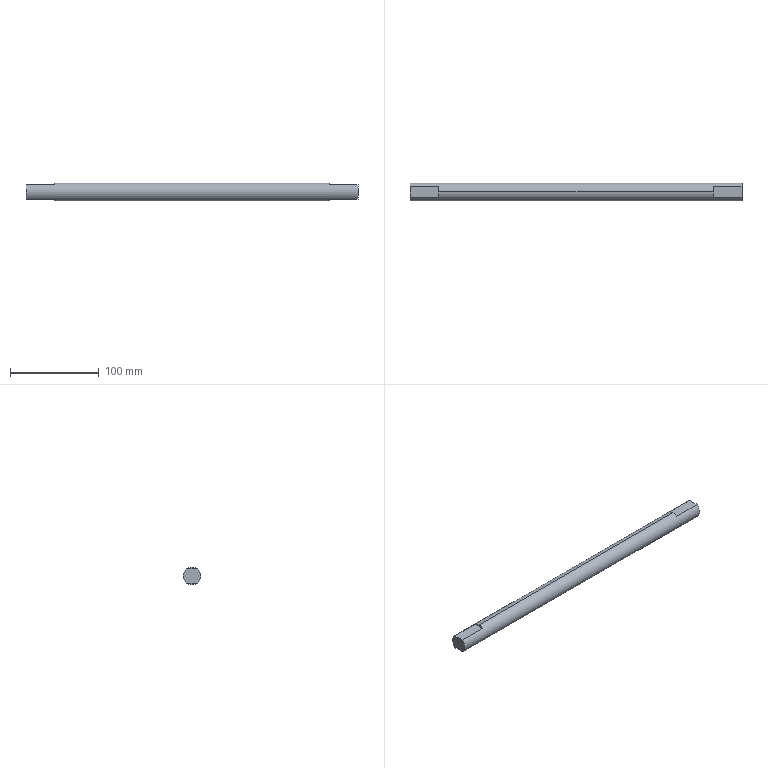Part | SolidWorks | features ICE 3, Extrusion 1, HoleWzd 1 | 1 solid | 12 faces | box 374 x 20 x 20 mm | volume 115370 mm3 | plane 10 | cylinder 2 | commonest cylinder face diameters 20 x2
STEP:
#1=CARTESIAN_POINT('',(341.5,6.,-8.));
#2=VERTEX_POINT('',#1);
#3=CARTESIAN_POINT('',(341.5,0.,-10.));
#4=VERTEX_POINT('',#3);
#5=CARTESIAN_POINT('',(341.5,0.,0.));
#6=DIRECTION('',(-1.,0.,0.));
#7=DIRECTION('',(0.,0.,1.));
#8=AXIS2_PLACEMENT_3D('',#5,#6,#7);
#9=CIRCLE('',#8,10.);
#10=EDGE_CURVE('',#2,#4,#9,.T.);
#11=ORIENTED_EDGE('',*,*,#10,.T.);
#12=CARTESIAN_POINT('',(32.5,0.,-10.));
#13=VERTEX_POINT('',#12);
#14=CARTESIAN_POINT('',(374.,0.,-10.));
#15=DIRECTION('',(-1.,0.,0.));
#16=VECTOR('',#15,1000.);
#17=LINE('',#14,#16);
#18=EDGE_CURVE('',#4,#13,#17,.T.);
#19=ORIENTED_EDGE('',*,*,#18,.T.);
#20=CARTESIAN_POINT('',(32.5,6.,-8.));
#21=VERTEX_POINT('',#20);
#22=CARTESIAN_POINT('',(32.5,0.,0.));
#23=DIRECTION('',(1.,0.,0.));
#24=DIRECTION('',(0.,1.,0.));
#25=AXIS2_PLACEMENT_3D('',#22,#23,#24);
#26=CIRCLE('',#25,10.);
#27=EDGE_CURVE('',#13,#21,#26,.T.);
#28=ORIENTED_EDGE('',*,*,#27,.T.);
#29=CARTESIAN_POINT('',(0.,6.,-8.));
#30=VERTEX_POINT('',#29);
#31=CARTESIAN_POINT('',(374.,6.,-8.));
#32=DIRECTION('',(-1.,0.,0.));
#33=VECTOR('',#32,1000.);
#34=LINE('',#31,#33);
#35=EDGE_CURVE('',#21,#30,#34,.T.);
#36=ORIENTED_EDGE('',*,*,#35,.T.);
#37=CARTESIAN_POINT('',(0.,6.,8.));
#38=VERTEX_POINT('',#37);
#39=CARTESIAN_POINT('',(0.,0.,0.));
#40=DIRECTION('',(1.,0.,0.));
#41=DIRECTION('',(0.,0.,-1.));
#42=AXIS2_PLACEMENT_3D('',#39,#40,#41);
#43=CIRCLE('',#42,10.);
#44=EDGE_CURVE('',#30,#38,#43,.T.);
#45=ORIENTED_EDGE('',*,*,#44,.T.);
#46=CARTESIAN_POINT('',(32.5,6.,8.));
#47=VERTEX_POINT('',#46);
#48=CARTESIAN_POINT('',(374.,6.,8.));
#49=DIRECTION('',(-1.,0.,0.));
#50=VECTOR('',#49,1000.);
#51=LINE('',#48,#50);
#52=EDGE_CURVE('',#47,#38,#51,.T.);
#53=ORIENTED_EDGE('',*,*,#52,.F.);
#54=CARTESIAN_POINT('',(32.5,0.,10.));
#55=VERTEX_POINT('',#54);
#56=CARTESIAN_POINT('',(32.5,0.,0.));
#57=DIRECTION('',(-1.,0.,0.));
#58=DIRECTION('',(0.,-1.,0.));
#59=AXIS2_PLACEMENT_3D('',#56,#57,#58);
#60=CIRCLE('',#59,10.);
#61=EDGE_CURVE('',#55,#47,#60,.T.);
#62=ORIENTED_EDGE('',*,*,#61,.F.);
#63=CARTESIAN_POINT('',(341.5,0.,10.));
#64=VERTEX_POINT('',#63);
#65=CARTESIAN_POINT('',(374.,0.,10.));
#66=DIRECTION('',(-1.,0.,0.));
#67=VECTOR('',#66,1000.);
#68=LINE('',#65,#67);
#69=EDGE_CURVE('',#64,#55,#68,.T.);
#70=ORIENTED_EDGE('',*,*,#69,.F.);
#71=CARTESIAN_POINT('',(341.5,6.,8.));
#72=VERTEX_POINT('',#71);
#73=CARTESIAN_POINT('',(341.5,0.,0.));
#74=DIRECTION('',(1.,0.,0.));
#75=DIRECTION('',(0.,0.,-1.));
#76=AXIS2_PLACEMENT_3D('',#73,#74,#75);
#77=CIRCLE('',#76,10.);
#78=EDGE_CURVE('',#72,#64,#77,.T.);
#79=ORIENTED_EDGE('',*,*,#78,.F.);
#80=CARTESIAN_POINT('',(374.,6.,8.));
#81=VERTEX_POINT('',#80);
#82=CARTESIAN_POINT('',(374.,6.,8.));
#83=DIRECTION('',(-1.,0.,0.));
#84=VECTOR('',#83,1000.);
#85=LINE('',#82,#84);
#86=EDGE_CURVE('',#81,#72,#85,.T.);
#87=ORIENTED_EDGE('',*,*,#86,.F.);
#88=CARTESIAN_POINT('',(374.,6.,-8.));
#89=VERTEX_POINT('',#88);
#90=CARTESIAN_POINT('',(374.,0.,0.));
#91=DIRECTION('',(1.,0.,0.));
#92=DIRECTION('',(0.,0.,-1.));
#93=AXIS2_PLACEMENT_3D('',#90,#91,#92);
#94=CIRCLE('',#93,10.);
#95=EDGE_CURVE('',#89,#81,#94,.T.);
#96=ORIENTED_EDGE('',*,*,#95,.F.);
#97=CARTESIAN_POINT('',(374.,6.,-8.));
#98=DIRECTION('',(-1.,0.,0.));
#99=VECTOR('',#98,1000.);
#100=LINE('',#97,#99);
#101=EDGE_CURVE('',#89,#2,#100,.T.);
#102=ORIENTED_EDGE('',*,*,#101,.T.);
#103=EDGE_LOOP('',(#11,#19,#28,#36,#45,#53,#62,#70,#79,#87,#96,#102));
#104=FACE_OUTER_BOUND('',#103,.T.);
#105=CARTESIAN_POINT('',(374.,0.,0.));
#106=DIRECTION('',(-1.,0.,0.));
#107=DIRECTION('',(0.,0.,1.));
#108=AXIS2_PLACEMENT_3D('',#105,#106,#107);
#109=CYLINDRICAL_SURFACE('',#108,10.);
#110=ADVANCED_FACE('',(#104),#109,.T.);
#111=ORIENTED_EDGE('',*,*,#18,.F.);
#112=CARTESIAN_POINT('',(341.5,-6.,-8.));
#113=VERTEX_POINT('',#112);
#114=CARTESIAN_POINT('',(341.5,0.,0.));
#115=DIRECTION('',(-1.,0.,0.));
#116=DIRECTION('',(0.,0.,1.));
#117=AXIS2_PLACEMENT_3D('',#114,#115,#116);
#118=CIRCLE('',#117,10.);
#119=EDGE_CURVE('',#4,#113,#118,.T.);
#120=ORIENTED_EDGE('',*,*,#119,.T.);
#121=CARTESIAN_POINT('',(374.,-6.,-8.));
#122=VERTEX_POINT('',#121);
#123=CARTESIAN_POINT('',(374.,-6.,-8.));
#124=DIRECTION('',(1.,0.,0.));
#125=VECTOR('',#124,1000.);
#126=LINE('',#123,#125);
#127=EDGE_CURVE('',#113,#122,#126,.T.);
#128=ORIENTED_EDGE('',*,*,#127,.T.);
#129=CARTESIAN_POINT('',(374.,-6.,8.));
#130=VERTEX_POINT('',#129);
#131=CARTESIAN_POINT('',(374.,0.,0.));
#132=DIRECTION('',(1.,0.,0.));
#133=DIRECTION('',(0.,0.,-1.));
#134=AXIS2_PLACEMENT_3D('',#131,#132,#133);
#135=CIRCLE('',#134,10.);
#136=EDGE_CURVE('',#130,#122,#135,.T.);
#137=ORIENTED_EDGE('',*,*,#136,.F.);
#138=CARTESIAN_POINT('',(341.5,-6.,8.));
#139=VERTEX_POINT('',#138);
#140=CARTESIAN_POINT('',(374.,-6.,8.));
#141=DIRECTION('',(1.,0.,0.));
#142=VECTOR('',#141,1000.);
#143=LINE('',#140,#142);
#144=EDGE_CURVE('',#139,#130,#143,.T.);
#145=ORIENTED_EDGE('',*,*,#144,.F.);
#146=CARTESIAN_POINT('',(341.5,0.,0.));
#147=DIRECTION('',(1.,0.,0.));
#148=DIRECTION('',(0.,0.,-1.));
#149=AXIS2_PLACEMENT_3D('',#146,#147,#148);
#150=CIRCLE('',#149,10.);
#151=EDGE_CURVE('',#64,#139,#150,.T.);
#152=ORIENTED_EDGE('',*,*,#151,.F.);
#153=ORIENTED_EDGE('',*,*,#69,.T.);
#154=CARTESIAN_POINT('',(32.5,-6.,8.));
#155=VERTEX_POINT('',#154);
#156=CARTESIAN_POINT('',(32.5,0.,0.));
#157=DIRECTION('',(-1.,0.,0.));
#158=DIRECTION('',(0.,-1.,0.));
#159=AXIS2_PLACEMENT_3D('',#156,#157,#158);
#160=CIRCLE('',#159,10.);
#161=EDGE_CURVE('',#155,#55,#160,.T.);
#162=ORIENTED_EDGE('',*,*,#161,.F.);
#163=CARTESIAN_POINT('',(0.,-6.,8.));
#164=VERTEX_POINT('',#163);
#165=CARTESIAN_POINT('',(374.,-6.,8.));
#166=DIRECTION('',(1.,0.,0.));
#167=VECTOR('',#166,1000.);
#168=LINE('',#165,#167);
#169=EDGE_CURVE('',#164,#155,#168,.T.);
#170=ORIENTED_EDGE('',*,*,#169,.F.);
#171=CARTESIAN_POINT('',(0.,-6.,-8.));
#172=VERTEX_POINT('',#171);
#173=CARTESIAN_POINT('',(0.,0.,0.));
#174=DIRECTION('',(1.,0.,0.));
#175=DIRECTION('',(0.,0.,-1.));
#176=AXIS2_PLACEMENT_3D('',#173,#174,#175);
#177=CIRCLE('',#176,10.);
#178=EDGE_CURVE('',#164,#172,#177,.T.);
#179=ORIENTED_EDGE('',*,*,#178,.T.);
#180=CARTESIAN_POINT('',(32.5,-6.,-8.));
#181=VERTEX_POINT('',#180);
#182=CARTESIAN_POINT('',(374.,-6.,-8.));
#183=DIRECTION('',(1.,0.,0.));
#184=VECTOR('',#183,1000.);
#185=LINE('',#182,#184);
#186=EDGE_CURVE('',#172,#181,#185,.T.);
#187=ORIENTED_EDGE('',*,*,#186,.T.);
#188=CARTESIAN_POINT('',(32.5,0.,0.));
#189=DIRECTION('',(1.,0.,0.));
#190=DIRECTION('',(0.,1.,0.));
#191=AXIS2_PLACEMENT_3D('',#188,#189,#190);
#192=CIRCLE('',#191,10.);
#193=EDGE_CURVE('',#181,#13,#192,.T.);
#194=ORIENTED_EDGE('',*,*,#193,.T.);
#195=EDGE_LOOP('',(#111,#120,#128,#137,#145,#152,#153,#162,#170,#179,#187,#194));
#196=FACE_OUTER_BOUND('',#195,.T.);
#197=CARTESIAN_POINT('',(374.,0.,0.));
#198=DIRECTION('',(-1.,0.,0.));
#199=DIRECTION('',(0.,0.,1.));
#200=AXIS2_PLACEMENT_3D('',#197,#198,#199);
#201=CYLINDRICAL_SURFACE('',#200,10.);
#202=ADVANCED_FACE('',(#196),#201,.T.);
#203=ORIENTED_EDGE('',*,*,#95,.T.);
#204=CARTESIAN_POINT('',(374.,0.,8.));
#205=DIRECTION('',(0.,-1.,0.));
#206=VECTOR('',#205,1000.);
#207=LINE('',#204,#206);
#208=EDGE_CURVE('',#81,#130,#207,.T.);
#209=ORIENTED_EDGE('',*,*,#208,.T.);
#210=ORIENTED_EDGE('',*,*,#136,.T.);
#211=CARTESIAN_POINT('',(374.,0.,-8.));
#212=DIRECTION('',(0.,-1.,0.));
#213=VECTOR('',#212,1000.);
#214=LINE('',#211,#213);
#215=EDGE_CURVE('',#89,#122,#214,.T.);
#216=ORIENTED_EDGE('',*,*,#215,.F.);
#217=EDGE_LOOP('',(#203,#209,#210,#216));
#218=FACE_OUTER_BOUND('',#217,.T.);
#219=CARTESIAN_POINT('',(374.,0.,0.));
#220=DIRECTION('',(1.,0.,0.));
#221=DIRECTION('',(0.,0.,-1.));
#222=AXIS2_PLACEMENT_3D('',#219,#220,#221);
#223=PLANE('',#222);
#224=ADVANCED_FACE('',(#218),#223,.T.);
#225=CARTESIAN_POINT('',(0.,0.,8.));
#226=DIRECTION('',(0.,-1.,0.));
#227=VECTOR('',#226,1000.);
#228=LINE('',#225,#227);
#229=EDGE_CURVE('',#38,#164,#228,.T.);
#230=ORIENTED_EDGE('',*,*,#229,.F.);
#231=ORIENTED_EDGE('',*,*,#44,.F.);
#232=CARTESIAN_POINT('',(0.,0.,-8.));
#233=DIRECTION('',(0.,-1.,0.));
#234=VECTOR('',#233,1000.);
#235=LINE('',#232,#234);
#236=EDGE_CURVE('',#30,#172,#235,.T.);
#237=ORIENTED_EDGE('',*,*,#236,.T.);
#238=ORIENTED_EDGE('',*,*,#178,.F.);
#239=EDGE_LOOP('',(#230,#231,#237,#238));
#240=FACE_OUTER_BOUND('',#239,.T.);
#241=CARTESIAN_POINT('',(0.,0.,0.));
#242=DIRECTION('',(1.,0.,0.));
#243=DIRECTION('',(0.,0.,-1.));
#244=AXIS2_PLACEMENT_3D('',#241,#242,#243);
#245=PLANE('',#244);
#246=ADVANCED_FACE('',(#240),#245,.F.);
#247=CARTESIAN_POINT('',(32.5,29.983,-8.));
#248=DIRECTION('',(0.,1.,0.));
#249=VECTOR('',#248,1000.);
#250=LINE('',#247,#249);
#251=EDGE_CURVE('',#181,#21,#250,.T.);
#252=ORIENTED_EDGE('',*,*,#251,.T.);
#253=ORIENTED_EDGE('',*,*,#27,.F.);
#254=ORIENTED_EDGE('',*,*,#193,.F.);
#255=EDGE_LOOP('',(#252,#253,#254));
#256=FACE_OUTER_BOUND('',#255,.T.);
#257=CARTESIAN_POINT('',(32.5,29.983,-28.));
#258=DIRECTION('',(1.,0.,0.));
#259=DIRECTION('',(0.,1.,0.));
#260=AXIS2_PLACEMENT_3D('',#257,#258,#259);
#261=PLANE('',#260);
#262=ADVANCED_FACE('',(#256),#261,.F.);
#263=ORIENTED_EDGE('',*,*,#251,.F.);
#264=ORIENTED_EDGE('',*,*,#186,.F.);
#265=ORIENTED_EDGE('',*,*,#236,.F.);
#266=ORIENTED_EDGE('',*,*,#35,.F.);
#267=EDGE_LOOP('',(#263,#264,#265,#266));
#268=FACE_OUTER_BOUND('',#267,.T.);
#269=CARTESIAN_POINT('',(0.,0.,-8.));
#270=DIRECTION('',(0.,0.,1.));
#271=DIRECTION('',(1.,0.,0.));
#272=AXIS2_PLACEMENT_3D('',#269,#270,#271);
#273=PLANE('',#272);
#274=ADVANCED_FACE('',(#268),#273,.F.);
#275=CARTESIAN_POINT('',(341.5,28.635,-8.));
#276=DIRECTION('',(0.,-1.,0.));
#277=VECTOR('',#276,1000.);
#278=LINE('',#275,#277);
#279=EDGE_CURVE('',#2,#113,#278,.T.);
#280=ORIENTED_EDGE('',*,*,#279,.T.);
#281=ORIENTED_EDGE('',*,*,#119,.F.);
#282=ORIENTED_EDGE('',*,*,#10,.F.);
#283=EDGE_LOOP('',(#280,#281,#282));
#284=FACE_OUTER_BOUND('',#283,.T.);
#285=CARTESIAN_POINT('',(341.5,28.635,-28.));
#286=DIRECTION('',(-1.,0.,0.));
#287=DIRECTION('',(0.,0.,1.));
#288=AXIS2_PLACEMENT_3D('',#285,#286,#287);
#289=PLANE('',#288);
#290=ADVANCED_FACE('',(#284),#289,.F.);
#291=ORIENTED_EDGE('',*,*,#215,.T.);
#292=ORIENTED_EDGE('',*,*,#127,.F.);
#293=ORIENTED_EDGE('',*,*,#279,.F.);
#294=ORIENTED_EDGE('',*,*,#101,.F.);
#295=EDGE_LOOP('',(#291,#292,#293,#294));
#296=FACE_OUTER_BOUND('',#295,.T.);
#297=CARTESIAN_POINT('',(0.,0.,-8.));
#298=DIRECTION('',(0.,0.,1.));
#299=DIRECTION('',(1.,0.,0.));
#300=AXIS2_PLACEMENT_3D('',#297,#298,#299);
#301=PLANE('',#300);
#302=ADVANCED_FACE('',(#296),#301,.F.);
#303=ORIENTED_EDGE('',*,*,#161,.T.);
#304=ORIENTED_EDGE('',*,*,#61,.T.);
#305=CARTESIAN_POINT('',(32.5,29.983,8.));
#306=DIRECTION('',(0.,1.,0.));
#307=VECTOR('',#306,1000.);
#308=LINE('',#305,#307);
#309=EDGE_CURVE('',#155,#47,#308,.T.);
#310=ORIENTED_EDGE('',*,*,#309,.F.);
#311=EDGE_LOOP('',(#303,#304,#310));
#312=FACE_OUTER_BOUND('',#311,.T.);
#313=CARTESIAN_POINT('',(32.5,29.983,28.));
#314=DIRECTION('',(-1.,0.,0.));
#315=DIRECTION('',(0.,-1.,0.));
#316=AXIS2_PLACEMENT_3D('',#313,#314,#315);
#317=PLANE('',#316);
#318=ADVANCED_FACE('',(#312),#317,.T.);
#319=ORIENTED_EDGE('',*,*,#52,.T.);
#320=ORIENTED_EDGE('',*,*,#229,.T.);
#321=ORIENTED_EDGE('',*,*,#169,.T.);
#322=ORIENTED_EDGE('',*,*,#309,.T.);
#323=EDGE_LOOP('',(#319,#320,#321,#322));
#324=FACE_OUTER_BOUND('',#323,.T.);
#325=CARTESIAN_POINT('',(0.,0.,8.));
#326=DIRECTION('',(0.,0.,1.));
#327=DIRECTION('',(1.,0.,0.));
#328=AXIS2_PLACEMENT_3D('',#325,#326,#327);
#329=PLANE('',#328);
#330=ADVANCED_FACE('',(#324),#329,.T.);
#331=ORIENTED_EDGE('',*,*,#78,.T.);
#332=ORIENTED_EDGE('',*,*,#151,.T.);
#333=CARTESIAN_POINT('',(341.5,28.635,8.));
#334=DIRECTION('',(0.,-1.,0.));
#335=VECTOR('',#334,1000.);
#336=LINE('',#333,#335);
#337=EDGE_CURVE('',#72,#139,#336,.T.);
#338=ORIENTED_EDGE('',*,*,#337,.F.);
#339=EDGE_LOOP('',(#331,#332,#338));
#340=FACE_OUTER_BOUND('',#339,.T.);
#341=CARTESIAN_POINT('',(341.5,28.635,28.));
#342=DIRECTION('',(1.,0.,0.));
#343=DIRECTION('',(0.,0.,-1.));
#344=AXIS2_PLACEMENT_3D('',#341,#342,#343);
#345=PLANE('',#344);
#346=ADVANCED_FACE('',(#340),#345,.T.);
#347=ORIENTED_EDGE('',*,*,#86,.T.);
#348=ORIENTED_EDGE('',*,*,#337,.T.);
#349=ORIENTED_EDGE('',*,*,#144,.T.);
#350=ORIENTED_EDGE('',*,*,#208,.F.);
#351=EDGE_LOOP('',(#347,#348,#349,#350));
#352=FACE_OUTER_BOUND('',#351,.T.);
#353=CARTESIAN_POINT('',(0.,0.,8.));
#354=DIRECTION('',(0.,0.,1.));
#355=DIRECTION('',(1.,0.,0.));
#356=AXIS2_PLACEMENT_3D('',#353,#354,#355);
#357=PLANE('',#356);
#358=ADVANCED_FACE('',(#352),#357,.T.);
#359=CLOSED_SHELL('',(#110,#202,#224,#246,#262,#274,#290,#302,#318,#330,#346,#358));
#360=MANIFOLD_SOLID_BREP('',#359);
#361=CARTESIAN_POINT('',(0.,0.,0.));
#362=DIRECTION('',(0.,0.,1.));
#363=DIRECTION('',(1.,0.,0.));
#364=AXIS2_PLACEMENT_3D('',#361,#362,#363);
#365=(LENGTH_UNIT()NAMED_UNIT(*)SI_UNIT(.MILLI.,.METRE.));
#366=UNCERTAINTY_MEASURE_WITH_UNIT(LENGTH_MEASURE(0.00001),#365,'','');
#367=(NAMED_UNIT(*)PLANE_ANGLE_UNIT()SI_UNIT($,.RADIAN.));
#368=(NAMED_UNIT(*)SI_UNIT($,.STERADIAN.)SOLID_ANGLE_UNIT());
#369=(GEOMETRIC_REPRESENTATION_CONTEXT(3)GLOBAL_UNCERTAINTY_ASSIGNED_CONTEXT((#366))GLOBAL_UNIT_ASSIGNED_CONTEXT((#365,#367,#368))REPRESENTATION_CONTEXT('',''));
#370=ADVANCED_BREP_SHAPE_REPRESENTATION('',(#360,#364),#369);